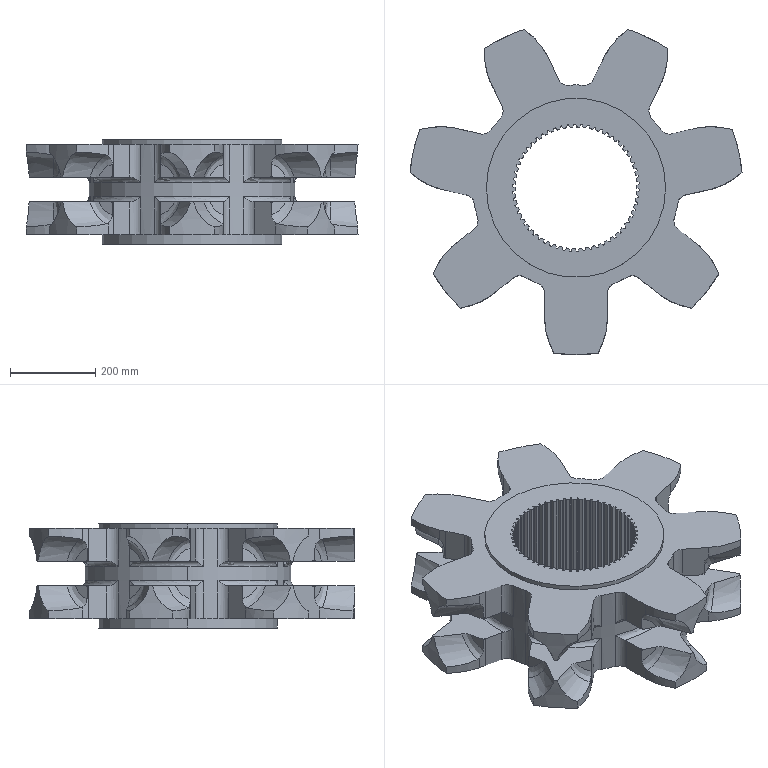Part | SolidWorks | features ICE 8, CirPattern 6, Fillet 3, MirrorPattern 2, 3DProfileFeature 1, BlendCut 1, Extrusion 1 | 1 solid | 556 faces | box 777.762 x 761.728 x 244 mm | volume 45916773 mm3 | spline 228 | cylinder 196 | plane 116 | torus 16 | commonest cylinder face diameters 285.1 x58 297.5 x58 48 x32 604.088 x28 781 x14 420 x4